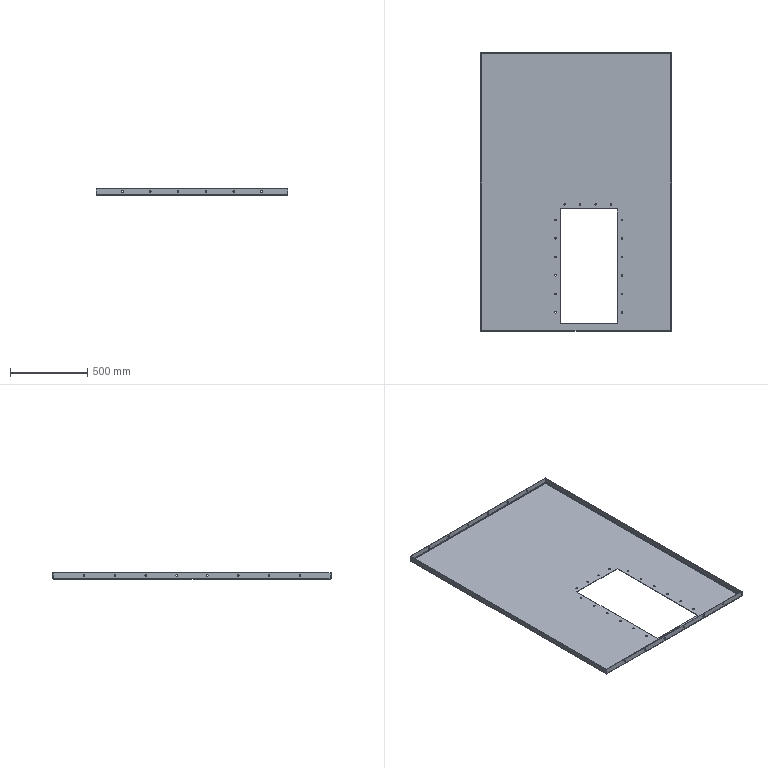Part | SolidWorks | features ICE 3, CornerFeat 1, EdgeFlange 1, FlatPattern 1, RefAxis 1, SMBaseFlange 1, SheetMetal 1 | 1 solid | 130 faces | box 1240 x 1800 x 40 mm | volume 6502410 mm3 | cylinder 96 | plane 26 | spline 8 | commonest cylinder face diameters 10 x88 6 x4 12 x4